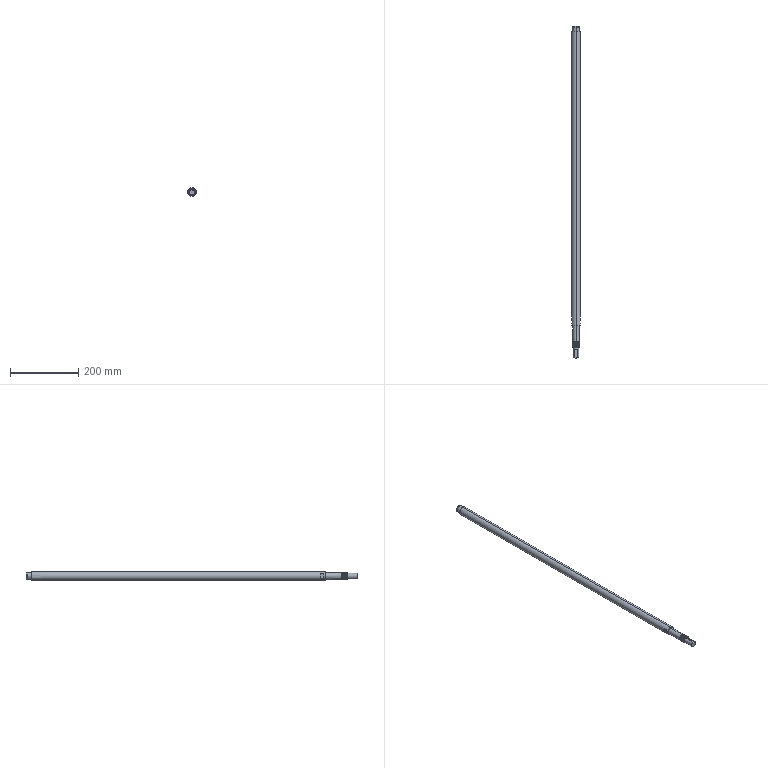Part | STEP file | 1 solid | 149 faces | box 25 x 970 x 25 mm | volume 453168 mm3 | cylinder 121 | plane 18 | cone 7 | spline 3 | commonest cylinder face diameters 20 x113 6 x2 17 x2 18.5 x2 25 x2